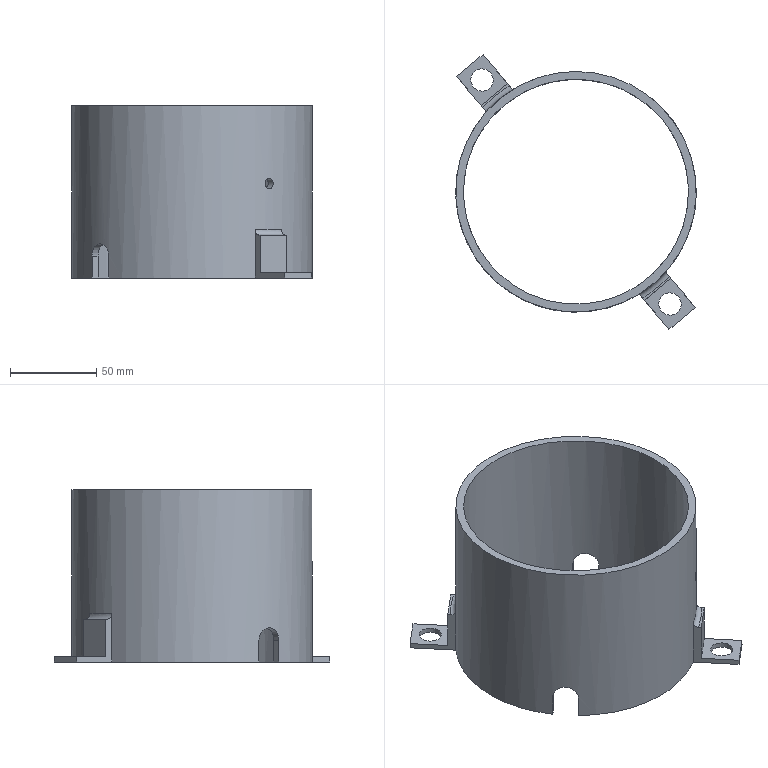Part | NX | features solid 2 | 1 solid | 30 faces | box 139.8 x 159.936 x 100 mm | volume 194922 mm3 | plane 21 | cylinder 7 | torus 2 | commonest cylinder face diameters 13 x2 15 x2 6 x1 130.8 x1 139.8 x1
STEP:
#1=CARTESIAN_POINT('',(1445.459,-595.134,-125.));
#2=VERTEX_POINT('',#1);
#3=CARTESIAN_POINT('',(1449.637,-600.114,-125.));
#4=DIRECTION('',(0.,0.,-1.));
#5=DIRECTION('',(-0.6428,0.766,0.));
#6=AXIS2_PLACEMENT_3D('',#3,#4,#5);
#7=CIRCLE('',#6,6.5);
#8=EDGE_CURVE('',#2,#2,#7,.T.);
#9=ORIENTED_EDGE('',*,*,#8,.F.);
#10=EDGE_LOOP('',(#9));
#11=FACE_BOUND('',#10,.T.);
#12=CARTESIAN_POINT('',(1453.058,-496.074,-125.));
#13=VERTEX_POINT('',#12);
#14=CARTESIAN_POINT('',(1447.129,-581.568,-125.));
#15=VERTEX_POINT('',#14);
#16=CARTESIAN_POINT('',(1395.,-535.,-125.));
#17=DIRECTION('',(0.,0.,-1.));
#18=DIRECTION('',(-0.9659,0.2588,0.));
#19=AXIS2_PLACEMENT_3D('',#16,#17,#18);
#20=CIRCLE('',#19,69.9);
#21=EDGE_CURVE('',#13,#15,#20,.T.);
#22=ORIENTED_EDGE('',*,*,#21,.T.);
#23=CARTESIAN_POINT('',(1464.368,-602.112,-125.));
#24=VERTEX_POINT('',#23);
#25=CARTESIAN_POINT('',(1437.371,-569.939,-125.));
#26=DIRECTION('',(0.6428,-0.766,0.));
#27=VECTOR('',#26,1000.);
#28=LINE('',#25,#27);
#29=EDGE_CURVE('',#15,#24,#28,.T.);
#30=ORIENTED_EDGE('',*,*,#29,.T.);
#31=CARTESIAN_POINT('',(1449.047,-614.968,-125.));
#32=VERTEX_POINT('',#31);
#33=CARTESIAN_POINT('',(1449.047,-614.968,-125.));
#34=DIRECTION('',(0.766,0.6428,0.));
#35=VECTOR('',#34,1000.);
#36=LINE('',#33,#35);
#37=EDGE_CURVE('',#32,#24,#36,.T.);
#38=ORIENTED_EDGE('',*,*,#37,.F.);
#39=CARTESIAN_POINT('',(1431.808,-594.424,-125.));
#40=VERTEX_POINT('',#39);
#41=CARTESIAN_POINT('',(1427.835,-589.689,-125.));
#42=DIRECTION('',(-0.6428,0.766,0.));
#43=VECTOR('',#42,1000.);
#44=LINE('',#41,#43);
#45=EDGE_CURVE('',#32,#40,#44,.T.);
#46=ORIENTED_EDGE('',*,*,#45,.T.);
#47=CARTESIAN_POINT('',(1346.584,-585.417,-125.));
#48=VERTEX_POINT('',#47);
#49=CARTESIAN_POINT('',(1395.,-535.,-125.));
#50=DIRECTION('',(0.,0.,-1.));
#51=DIRECTION('',(-0.9659,0.2588,0.));
#52=AXIS2_PLACEMENT_3D('',#49,#50,#51);
#53=CIRCLE('',#52,69.9);
#54=EDGE_CURVE('',#40,#48,#53,.T.);
#55=ORIENTED_EDGE('',*,*,#54,.T.);
#56=CARTESIAN_POINT('',(1350.052,-582.506,-125.));
#57=VERTEX_POINT('',#56);
#58=CARTESIAN_POINT('',(1399.821,-540.745,-125.));
#59=DIRECTION('',(-0.766,-0.6428,0.));
#60=VECTOR('',#59,1000.);
#61=LINE('',#58,#60);
#62=EDGE_CURVE('',#57,#48,#61,.T.);
#63=ORIENTED_EDGE('',*,*,#62,.F.);
#64=CARTESIAN_POINT('',(1449.59,-498.984,-125.));
#65=VERTEX_POINT('',#64);
#66=CARTESIAN_POINT('',(1395.,-535.,-125.));
#67=DIRECTION('',(0.,0.,-1.));
#68=DIRECTION('',(-0.9659,0.2588,0.));
#69=AXIS2_PLACEMENT_3D('',#66,#67,#68);
#70=CIRCLE('',#69,65.4);
#71=EDGE_CURVE('',#65,#57,#70,.T.);
#72=ORIENTED_EDGE('',*,*,#71,.F.);
#73=CARTESIAN_POINT('',(1399.821,-540.745,-125.));
#74=DIRECTION('',(-0.766,-0.6428,0.));
#75=VECTOR('',#74,1000.);
#76=LINE('',#73,#75);
#77=EDGE_CURVE('',#13,#65,#76,.T.);
#78=ORIENTED_EDGE('',*,*,#77,.F.);
#79=EDGE_LOOP('',(#22,#30,#38,#46,#55,#63,#72,#78));
#80=FACE_BOUND('',#79,.T.);
#81=CARTESIAN_POINT('',(1395.,-535.,-125.));
#82=DIRECTION('',(0.,0.,1.));
#83=DIRECTION('',(-0.6428,0.766,0.));
#84=AXIS2_PLACEMENT_3D('',#81,#82,#83);
#85=PLANE('',#84);
#86=ADVANCED_FACE('',(#11,#80),#85,.F.);
#87=CARTESIAN_POINT('',(1355.094,-471.885,-100.));
#88=VERTEX_POINT('',#87);
#89=CARTESIAN_POINT('',(1356.244,-473.255,-100.));
#90=VERTEX_POINT('',#89);
#91=CARTESIAN_POINT('',(1362.165,-480.311,-100.));
#92=DIRECTION('',(0.6428,-0.766,0.));
#93=VECTOR('',#92,1000.);
#94=LINE('',#91,#93);
#95=EDGE_CURVE('',#88,#90,#94,.T.);
#96=ORIENTED_EDGE('',*,*,#95,.F.);
#97=CARTESIAN_POINT('',(1347.434,-478.313,-100.));
#98=VERTEX_POINT('',#97);
#99=CARTESIAN_POINT('',(1339.773,-484.741,-100.));
#100=DIRECTION('',(0.766,0.6428,0.));
#101=VECTOR('',#100,1000.);
#102=LINE('',#99,#101);
#103=EDGE_CURVE('',#98,#88,#102,.T.);
#104=ORIENTED_EDGE('',*,*,#103,.F.);
#105=CARTESIAN_POINT('',(1348.141,-479.155,-100.));
#106=VERTEX_POINT('',#105);
#107=CARTESIAN_POINT('',(1348.141,-479.155,-100.));
#108=CARTESIAN_POINT('',(1347.905,-478.874,-100.));
#109=CARTESIAN_POINT('',(1347.669,-478.594,-100.));
#110=CARTESIAN_POINT('',(1347.434,-478.313,-100.));
#111=B_SPLINE_CURVE_WITH_KNOTS('',3,(#107,#108,#109,#110),.UNSPECIFIED.,.F.,.F.,(4,4),(0.9,1.),.UNSPECIFIED.);
#112=EDGE_CURVE('',#106,#98,#111,.T.);
#113=ORIENTED_EDGE('',*,*,#112,.F.);
#114=CARTESIAN_POINT('',(1395.,-535.,-100.));
#115=DIRECTION('',(0.,0.,-1.));
#116=DIRECTION('',(-0.9659,0.2588,0.));
#117=AXIS2_PLACEMENT_3D('',#114,#115,#116);
#118=CIRCLE('',#117,72.9);
#119=EDGE_CURVE('',#90,#106,#118,.F.);
#120=ORIENTED_EDGE('',*,*,#119,.F.);
#121=EDGE_LOOP('',(#96,#104,#113,#120));
#122=FACE_BOUND('',#121,.T.);
#123=CARTESIAN_POINT('',(1367.95,-487.206,-100.));
#124=DIRECTION('',(0.,0.,1.));
#125=DIRECTION('',(-0.6428,0.766,0.));
#126=AXIS2_PLACEMENT_3D('',#123,#124,#125);
#127=PLANE('',#126);
#128=ADVANCED_FACE('',(#122),#127,.T.);
#129=CARTESIAN_POINT('',(1434.906,-598.115,-100.));
#130=VERTEX_POINT('',#129);
#131=CARTESIAN_POINT('',(1433.756,-596.745,-100.));
#132=VERTEX_POINT('',#131);
#133=CARTESIAN_POINT('',(1427.835,-589.689,-100.));
#134=DIRECTION('',(-0.6428,0.766,0.));
#135=VECTOR('',#134,1000.);
#136=LINE('',#133,#135);
#137=EDGE_CURVE('',#130,#132,#136,.T.);
#138=ORIENTED_EDGE('',*,*,#137,.F.);
#139=CARTESIAN_POINT('',(1442.566,-591.687,-100.));
#140=VERTEX_POINT('',#139);
#141=CARTESIAN_POINT('',(1450.227,-585.259,-100.));
#142=DIRECTION('',(-0.766,-0.6428,0.));
#143=VECTOR('',#142,1000.);
#144=LINE('',#141,#143);
#145=EDGE_CURVE('',#140,#130,#144,.T.);
#146=ORIENTED_EDGE('',*,*,#145,.F.);
#147=CARTESIAN_POINT('',(1441.859,-590.845,-100.));
#148=VERTEX_POINT('',#147);
#149=CARTESIAN_POINT('',(1441.859,-590.845,-100.));
#150=CARTESIAN_POINT('',(1442.095,-591.126,-100.));
#151=CARTESIAN_POINT('',(1442.331,-591.406,-100.));
#152=CARTESIAN_POINT('',(1442.566,-591.687,-100.));
#153=B_SPLINE_CURVE_WITH_KNOTS('',3,(#149,#150,#151,#152),.UNSPECIFIED.,.F.,.F.,(4,4),(0.9,1.),.UNSPECIFIED.);
#154=EDGE_CURVE('',#148,#140,#153,.T.);
#155=ORIENTED_EDGE('',*,*,#154,.F.);
#156=CARTESIAN_POINT('',(1395.,-535.,-100.));
#157=DIRECTION('',(0.,0.,-1.));
#158=DIRECTION('',(-0.9659,0.2588,0.));
#159=AXIS2_PLACEMENT_3D('',#156,#157,#158);
#160=CIRCLE('',#159,72.9);
#161=EDGE_CURVE('',#132,#148,#160,.F.);
#162=ORIENTED_EDGE('',*,*,#161,.F.);
#163=EDGE_LOOP('',(#138,#146,#155,#162));
#164=FACE_BOUND('',#163,.T.);
#165=CARTESIAN_POINT('',(1427.835,-589.689,-100.));
#166=DIRECTION('',(0.,0.,1.));
#167=DIRECTION('',(-0.6428,0.766,0.));
#168=AXIS2_PLACEMENT_3D('',#165,#166,#167);
#169=PLANE('',#168);
#170=ADVANCED_FACE('',(#164),#169,.T.);
#171=CARTESIAN_POINT('',(1439.646,-588.784,-72.977));
#172=VERTEX_POINT('',#171);
#173=CARTESIAN_POINT('',(1437.891,-590.2,-72.04));
#174=CARTESIAN_POINT('',(1439.626,-588.821,-73.3));
#175=CARTESIAN_POINT('',(1441.483,-587.218,-72.622));
#176=CARTESIAN_POINT('',(1442.407,-586.366,-70.413));
#177=CARTESIAN_POINT('',(1441.913,-586.826,-67.959));
#178=CARTESIAN_POINT('',(1440.255,-588.293,-66.701));
#179=CARTESIAN_POINT('',(1438.356,-589.842,-67.375));
#180=CARTESIAN_POINT('',(1437.353,-590.606,-69.586));
#181=CARTESIAN_POINT('',(1437.891,-590.2,-72.04));
#182=CARTESIAN_POINT('',(1439.626,-588.821,-73.3));
#183=CARTESIAN_POINT('',(1441.483,-587.218,-72.622));
#184=B_SPLINE_CURVE_WITH_KNOTS('',3,(#173,#174,#175,#176,#177,#178,#179,#180,#181,#182,#183),.UNSPECIFIED.,.T.,.F.,(1,1,1,1,1,1,1,1,1,1,1,1,1,1,1),(-0.007035,-0.00469,-0.002345,0.,0.002345,0.00469,0.007035,0.009379,0.01172,0.01407,0.01641,0.01876,0.0211,0.02345,0.02579),.UNSPECIFIED.);
#185=EDGE_CURVE('',#172,#172,#184,.T.);
#186=ORIENTED_EDGE('',*,*,#185,.F.);
#187=EDGE_LOOP('',(#186));
#188=FACE_BOUND('',#187,.T.);
#189=CARTESIAN_POINT('',(1327.482,-516.909,-25.));
#190=VERTEX_POINT('',#189);
#191=CARTESIAN_POINT('',(1395.,-535.,-25.));
#192=DIRECTION('',(0.,0.,-1.));
#193=DIRECTION('',(-0.9659,0.2588,0.));
#194=AXIS2_PLACEMENT_3D('',#191,#192,#193);
#195=CIRCLE('',#194,69.9);
#196=EDGE_CURVE('',#190,#190,#195,.T.);
#197=ORIENTED_EDGE('',*,*,#196,.T.);
#198=EDGE_LOOP('',(#197));
#199=FACE_BOUND('',#198,.T.);
#200=CARTESIAN_POINT('',(1443.416,-484.583,-112.5));
#201=VERTEX_POINT('',#200);
#202=CARTESIAN_POINT('',(1453.058,-496.074,-112.5));
#203=VERTEX_POINT('',#202);
#204=CARTESIAN_POINT('',(1443.416,-484.583,-112.5));
#205=CARTESIAN_POINT('',(1443.416,-484.583,-110.517));
#206=CARTESIAN_POINT('',(1444.616,-485.698,-106.634));
#207=CARTESIAN_POINT('',(1448.619,-489.999,-104.184));
#208=CARTESIAN_POINT('',(1452.168,-494.697,-106.628));
#209=CARTESIAN_POINT('',(1453.058,-496.074,-110.517));
#210=CARTESIAN_POINT('',(1453.058,-496.074,-112.5));
#211=B_SPLINE_CURVE_WITH_KNOTS('',3,(#204,#205,#206,#207,#208,#209,#210),.UNSPECIFIED.,.F.,.F.,(4,1,1,1,4),(0.,0.005865,0.01173,0.0176,0.02346),.UNSPECIFIED.);
#212=EDGE_CURVE('',#201,#203,#211,.T.);
#213=ORIENTED_EDGE('',*,*,#212,.F.);
#214=CARTESIAN_POINT('',(1443.416,-484.583,-125.));
#215=VERTEX_POINT('',#214);
#216=CARTESIAN_POINT('',(1443.416,-484.583,-118.75));
#217=DIRECTION('',(0.,0.,-1.));
#218=VECTOR('',#217,1000.);
#219=LINE('',#216,#218);
#220=EDGE_CURVE('',#215,#201,#219,.F.);
#221=ORIENTED_EDGE('',*,*,#220,.F.);
#222=CARTESIAN_POINT('',(1358.192,-475.576,-125.));
#223=VERTEX_POINT('',#222);
#224=CARTESIAN_POINT('',(1395.,-535.,-125.));
#225=DIRECTION('',(0.,0.,-1.));
#226=DIRECTION('',(-0.9659,0.2588,0.));
#227=AXIS2_PLACEMENT_3D('',#224,#225,#226);
#228=CIRCLE('',#227,69.9);
#229=EDGE_CURVE('',#223,#215,#228,.T.);
#230=ORIENTED_EDGE('',*,*,#229,.F.);
#231=CARTESIAN_POINT('',(1358.192,-475.576,-97.));
#232=VERTEX_POINT('',#231);
#233=CARTESIAN_POINT('',(1358.192,-475.576,-111.));
#234=DIRECTION('',(0.,0.,-1.));
#235=VECTOR('',#234,1000.);
#236=LINE('',#233,#235);
#237=EDGE_CURVE('',#223,#232,#236,.F.);
#238=ORIENTED_EDGE('',*,*,#237,.T.);
#239=CARTESIAN_POINT('',(1342.871,-488.432,-97.));
#240=VERTEX_POINT('',#239);
#241=CARTESIAN_POINT('',(1395.,-535.,-97.));
#242=DIRECTION('',(0.,0.,-1.));
#243=DIRECTION('',(-0.9659,0.2588,0.));
#244=AXIS2_PLACEMENT_3D('',#241,#242,#243);
#245=CIRCLE('',#244,69.9);
#246=EDGE_CURVE('',#240,#232,#245,.T.);
#247=ORIENTED_EDGE('',*,*,#246,.F.);
#248=CARTESIAN_POINT('',(1342.871,-488.432,-125.));
#249=VERTEX_POINT('',#248);
#250=CARTESIAN_POINT('',(1342.871,-488.432,-111.));
#251=DIRECTION('',(0.,0.,-1.));
#252=VECTOR('',#251,1000.);
#253=LINE('',#250,#252);
#254=EDGE_CURVE('',#240,#249,#253,.T.);
#255=ORIENTED_EDGE('',*,*,#254,.T.);
#256=CARTESIAN_POINT('',(1336.942,-573.926,-125.));
#257=VERTEX_POINT('',#256);
#258=CARTESIAN_POINT('',(1395.,-535.,-125.));
#259=DIRECTION('',(0.,0.,-1.));
#260=DIRECTION('',(-0.9659,0.2588,0.));
#261=AXIS2_PLACEMENT_3D('',#258,#259,#260);
#262=CIRCLE('',#261,69.9);
#263=EDGE_CURVE('',#257,#249,#262,.T.);
#264=ORIENTED_EDGE('',*,*,#263,.F.);
#265=CARTESIAN_POINT('',(1336.942,-573.926,-112.5));
#266=VERTEX_POINT('',#265);
#267=CARTESIAN_POINT('',(1336.942,-573.926,-118.75));
#268=DIRECTION('',(0.,0.,-1.));
#269=VECTOR('',#268,1000.);
#270=LINE('',#267,#269);
#271=EDGE_CURVE('',#266,#257,#270,.T.);
#272=ORIENTED_EDGE('',*,*,#271,.F.);
#273=CARTESIAN_POINT('',(1346.584,-585.417,-112.5));
#274=VERTEX_POINT('',#273);
#275=CARTESIAN_POINT('',(1346.584,-585.417,-112.5));
#276=CARTESIAN_POINT('',(1346.584,-585.417,-110.517));
#277=CARTESIAN_POINT('',(1345.384,-584.302,-106.634));
#278=CARTESIAN_POINT('',(1341.381,-580.001,-104.184));
#279=CARTESIAN_POINT('',(1337.832,-575.303,-106.628));
#280=CARTESIAN_POINT('',(1336.942,-573.926,-110.517));
#281=CARTESIAN_POINT('',(1336.942,-573.926,-112.5));
#282=B_SPLINE_CURVE_WITH_KNOTS('',3,(#275,#276,#277,#278,#279,#280,#281),.UNSPECIFIED.,.F.,.F.,(4,1,1,1,4),(0.,0.005865,0.01173,0.0176,0.02346),.UNSPECIFIED.);
#283=EDGE_CURVE('',#274,#266,#282,.T.);
#284=ORIENTED_EDGE('',*,*,#283,.F.);
#285=CARTESIAN_POINT('',(1346.584,-585.417,-118.75));
#286=DIRECTION('',(0.,0.,-1.));
#287=VECTOR('',#286,1000.);
#288=LINE('',#285,#287);
#289=EDGE_CURVE('',#48,#274,#288,.F.);
#290=ORIENTED_EDGE('',*,*,#289,.F.);
#291=ORIENTED_EDGE('',*,*,#54,.F.);
#292=CARTESIAN_POINT('',(1431.808,-594.424,-97.));
#293=VERTEX_POINT('',#292);
#294=CARTESIAN_POINT('',(1431.808,-594.424,-111.));
#295=DIRECTION('',(0.,0.,-1.));
#296=VECTOR('',#295,1000.);
#297=LINE('',#294,#296);
#298=EDGE_CURVE('',#40,#293,#297,.F.);
#299=ORIENTED_EDGE('',*,*,#298,.T.);
#300=CARTESIAN_POINT('',(1447.129,-581.568,-97.));
#301=VERTEX_POINT('',#300);
#302=CARTESIAN_POINT('',(1395.,-535.,-97.));
#303=DIRECTION('',(0.,0.,-1.));
#304=DIRECTION('',(-0.9659,0.2588,0.));
#305=AXIS2_PLACEMENT_3D('',#302,#303,#304);
#306=CIRCLE('',#305,69.9);
#307=EDGE_CURVE('',#301,#293,#306,.T.);
#308=ORIENTED_EDGE('',*,*,#307,.F.);
#309=CARTESIAN_POINT('',(1447.129,-581.568,-111.));
#310=DIRECTION('',(0.,0.,-1.));
#311=VECTOR('',#310,1000.);
#312=LINE('',#309,#311);
#313=EDGE_CURVE('',#301,#15,#312,.T.);
#314=ORIENTED_EDGE('',*,*,#313,.T.);
#315=ORIENTED_EDGE('',*,*,#21,.F.);
#316=CARTESIAN_POINT('',(1453.058,-496.074,-118.75));
#317=DIRECTION('',(0.,0.,-1.));
#318=VECTOR('',#317,1000.);
#319=LINE('',#316,#318);
#320=EDGE_CURVE('',#203,#13,#319,.T.);
#321=ORIENTED_EDGE('',*,*,#320,.F.);
#322=EDGE_LOOP('',(#213,#221,#230,#238,#247,#255,#264,#272,#284,#290,#291,#299,#308,#314,#315,#321));
#323=FACE_BOUND('',#322,.T.);
#324=CARTESIAN_POINT('',(1395.,-535.,-15.));
#325=DIRECTION('',(0.,0.,-1.));
#326=DIRECTION('',(0.6428,-0.766,0.));
#327=AXIS2_PLACEMENT_3D('',#324,#325,#326);
#328=CYLINDRICAL_SURFACE('',#327,69.9);
#329=ADVANCED_FACE('',(#188,#199,#323),#328,.T.);
#330=CARTESIAN_POINT('',(1449.59,-498.984,-112.5));
#331=VERTEX_POINT('',#330);
#332=CARTESIAN_POINT('',(1449.59,-498.984,-118.75));
#333=DIRECTION('',(0.,0.,-1.));
#334=VECTOR('',#333,1000.);
#335=LINE('',#332,#334);
#336=EDGE_CURVE('',#331,#65,#335,.T.);
#337=ORIENTED_EDGE('',*,*,#336,.T.);
#338=ORIENTED_EDGE('',*,*,#71,.T.);
#339=CARTESIAN_POINT('',(1350.052,-582.506,-112.5));
#340=VERTEX_POINT('',#339);
#341=CARTESIAN_POINT('',(1350.052,-582.506,-118.75));
#342=DIRECTION('',(0.,0.,-1.));
#343=VECTOR('',#342,1000.);
#344=LINE('',#341,#343);
#345=EDGE_CURVE('',#57,#340,#344,.F.);
#346=ORIENTED_EDGE('',*,*,#345,.T.);
#347=CARTESIAN_POINT('',(1340.41,-571.016,-112.5));
#348=VERTEX_POINT('',#347);
#349=CARTESIAN_POINT('',(1350.052,-582.506,-112.5));
#350=CARTESIAN_POINT('',(1350.052,-582.506,-110.517));
#351=CARTESIAN_POINT('',(1348.842,-581.4,-106.634));
#352=CARTESIAN_POINT('',(1344.823,-577.113,-104.184));
#353=CARTESIAN_POINT('',(1341.29,-572.401,-106.629));
#354=CARTESIAN_POINT('',(1340.41,-571.016,-110.517));
#355=CARTESIAN_POINT('',(1340.41,-571.016,-112.5));
#356=B_SPLINE_CURVE_WITH_KNOTS('',3,(#349,#350,#351,#352,#353,#354,#355),.UNSPECIFIED.,.F.,.F.,(4,1,1,1,4),(0.,0.005866,0.01173,0.0176,0.02346),.UNSPECIFIED.);
#357=EDGE_CURVE('',#340,#348,#356,.T.);
#358=ORIENTED_EDGE('',*,*,#357,.T.);
#359=CARTESIAN_POINT('',(1340.41,-571.016,-125.));
#360=VERTEX_POINT('',#359);
#361=CARTESIAN_POINT('',(1340.41,-571.016,-118.75));
#362=DIRECTION('',(0.,0.,-1.));
#363=VECTOR('',#362,1000.);
#364=LINE('',#361,#363);
#365=EDGE_CURVE('',#348,#360,#364,.T.);
#366=ORIENTED_EDGE('',*,*,#365,.T.);
#367=CARTESIAN_POINT('',(1439.948,-487.494,-125.));
#368=VERTEX_POINT('',#367);
#369=CARTESIAN_POINT('',(1395.,-535.,-125.));
#370=DIRECTION('',(0.,0.,-1.));
#371=DIRECTION('',(-0.9659,0.2588,0.));
#372=AXIS2_PLACEMENT_3D('',#369,#370,#371);
#373=CIRCLE('',#372,65.4);
#374=EDGE_CURVE('',#360,#368,#373,.T.);
#375=ORIENTED_EDGE('',*,*,#374,.T.);
#376=CARTESIAN_POINT('',(1439.948,-487.494,-112.5));
#377=VERTEX_POINT('',#376);
#378=CARTESIAN_POINT('',(1439.948,-487.494,-118.75));
#379=DIRECTION('',(0.,0.,-1.));
#380=VECTOR('',#379,1000.);
#381=LINE('',#378,#380);
#382=EDGE_CURVE('',#368,#377,#381,.F.);
#383=ORIENTED_EDGE('',*,*,#382,.T.);
#384=CARTESIAN_POINT('',(1439.948,-487.494,-112.5));
#385=CARTESIAN_POINT('',(1439.948,-487.494,-110.517));
#386=CARTESIAN_POINT('',(1441.158,-488.6,-106.634));
#387=CARTESIAN_POINT('',(1445.177,-492.887,-104.184));
#388=CARTESIAN_POINT('',(1448.71,-497.599,-106.629));
#389=CARTESIAN_POINT('',(1449.59,-498.984,-110.517));
#390=CARTESIAN_POINT('',(1449.59,-498.984,-112.5));
#391=B_SPLINE_CURVE_WITH_KNOTS('',3,(#384,#385,#386,#387,#388,#389,#390),.UNSPECIFIED.,.F.,.F.,(4,1,1,1,4),(0.,0.005866,0.01173,0.0176,0.02346),.UNSPECIFIED.);
#392=EDGE_CURVE('',#377,#331,#391,.T.);
#393=ORIENTED_EDGE('',*,*,#392,.T.);
#394=EDGE_LOOP('',(#337,#338,#346,#358,#366,#375,#383,#393));
#395=FACE_BOUND('',#394,.T.);
#396=CARTESIAN_POINT('',(1436.742,-585.347,-72.975));
#397=VERTEX_POINT('',#396);
#398=CARTESIAN_POINT('',(1434.988,-586.757,-72.027));
#399=CARTESIAN_POINT('',(1436.721,-585.386,-73.298));
#400=CARTESIAN_POINT('',(1438.579,-583.779,-72.633));
#401=CARTESIAN_POINT('',(1439.509,-582.916,-70.43));
#402=CARTESIAN_POINT('',(1439.026,-583.369,-67.972));
#403=CARTESIAN_POINT('',(1437.376,-584.836,-66.703));
#404=CARTESIAN_POINT('',(1435.473,-586.385,-67.364));
#405=CARTESIAN_POINT('',(1434.459,-587.154,-69.569));
#406=CARTESIAN_POINT('',(1434.988,-586.757,-72.027));
#407=CARTESIAN_POINT('',(1436.721,-585.386,-73.298));
#408=CARTESIAN_POINT('',(1438.579,-583.779,-72.633));
#409=B_SPLINE_CURVE_WITH_KNOTS('',3,(#398,#399,#400,#401,#402,#403,#404,#405,#406,#407,#408),.UNSPECIFIED.,.T.,.F.,(1,1,1,1,1,1,1,1,1,1,1,1,1,1,1),(-0.007035,-0.00469,-0.002345,0.,0.002345,0.00469,0.007035,0.00938,0.01172,0.01407,0.01641,0.01876,0.0211,0.02345,0.02579),.UNSPECIFIED.);
#410=EDGE_CURVE('',#397,#397,#409,.T.);
#411=ORIENTED_EDGE('',*,*,#410,.T.);
#412=EDGE_LOOP('',(#411));
#413=FACE_BOUND('',#412,.T.);
#414=CARTESIAN_POINT('',(1331.828,-518.073,-25.));
#415=VERTEX_POINT('',#414);
#416=CARTESIAN_POINT('',(1395.,-535.,-25.));
#417=DIRECTION('',(0.,0.,-1.));
#418=DIRECTION('',(-0.9659,0.2588,0.));
#419=AXIS2_PLACEMENT_3D('',#416,#417,#418);
#420=CIRCLE('',#419,65.4);
#421=EDGE_CURVE('',#415,#415,#420,.T.);
#422=ORIENTED_EDGE('',*,*,#421,.F.);
#423=EDGE_LOOP('',(#422));
#424=FACE_BOUND('',#423,.T.);
#425=CARTESIAN_POINT('',(1395.,-535.,-15.));
#426=DIRECTION('',(0.,0.,-1.));
#427=DIRECTION('',(0.6428,-0.766,0.));
#428=AXIS2_PLACEMENT_3D('',#425,#426,#427);
#429=CYLINDRICAL_SURFACE('',#428,65.4);
#430=ADVANCED_FACE('',(#395,#413,#424),#429,.F.);
#431=ORIENTED_EDGE('',*,*,#421,.T.);
#432=EDGE_LOOP('',(#431));
#433=FACE_BOUND('',#432,.T.);
#434=ORIENTED_EDGE('',*,*,#196,.F.);
#435=EDGE_LOOP('',(#434));
#436=FACE_BOUND('',#435,.T.);
#437=CARTESIAN_POINT('',(1395.,-535.,-25.));
#438=DIRECTION('',(0.,0.,1.));
#439=DIRECTION('',(-0.6428,0.766,0.));
#440=AXIS2_PLACEMENT_3D('',#437,#438,#439);
#441=PLANE('',#440);
#442=ADVANCED_FACE('',(#433,#436),#441,.T.);
#443=ORIENTED_EDGE('',*,*,#374,.F.);
#444=CARTESIAN_POINT('',(1390.179,-529.255,-125.));
#445=DIRECTION('',(0.766,0.6428,0.));
#446=VECTOR('',#445,1000.);
#447=LINE('',#444,#446);
#448=EDGE_CURVE('',#257,#360,#447,.T.);
#449=ORIENTED_EDGE('',*,*,#448,.F.);
#450=ORIENTED_EDGE('',*,*,#263,.T.);
#451=CARTESIAN_POINT('',(1325.632,-467.888,-125.));
#452=VERTEX_POINT('',#451);
#453=CARTESIAN_POINT('',(1352.629,-500.061,-125.));
#454=DIRECTION('',(-0.6428,0.766,0.));
#455=VECTOR('',#454,1000.);
#456=LINE('',#453,#455);
#457=EDGE_CURVE('',#249,#452,#456,.T.);
#458=ORIENTED_EDGE('',*,*,#457,.T.);
#459=CARTESIAN_POINT('',(1340.953,-455.032,-125.));
#460=VERTEX_POINT('',#459);
#461=CARTESIAN_POINT('',(1340.953,-455.032,-125.));
#462=DIRECTION('',(-0.766,-0.6428,0.));
#463=VECTOR('',#462,1000.);
#464=LINE('',#461,#463);
#465=EDGE_CURVE('',#460,#452,#464,.T.);
#466=ORIENTED_EDGE('',*,*,#465,.F.);
#467=CARTESIAN_POINT('',(1362.165,-480.311,-125.));
#468=DIRECTION('',(0.6428,-0.766,0.));
#469=VECTOR('',#468,1000.);
#470=LINE('',#467,#469);
#471=EDGE_CURVE('',#460,#223,#470,.T.);
#472=ORIENTED_EDGE('',*,*,#471,.T.);
#473=ORIENTED_EDGE('',*,*,#229,.T.);
#474=CARTESIAN_POINT('',(1390.179,-529.255,-125.));
#475=DIRECTION('',(0.766,0.6428,0.));
#476=VECTOR('',#475,1000.);
#477=LINE('',#474,#476);
#478=EDGE_CURVE('',#368,#215,#477,.T.);
#479=ORIENTED_EDGE('',*,*,#478,.F.);
#480=EDGE_LOOP('',(#443,#449,#450,#458,#466,#472,#473,#479));
#481=FACE_BOUND('',#480,.T.);
#482=CARTESIAN_POINT('',(1336.185,-464.907,-125.));
#483=VERTEX_POINT('',#482);
#484=CARTESIAN_POINT('',(1340.363,-469.886,-125.));
#485=DIRECTION('',(0.,0.,-1.));
#486=DIRECTION('',(-0.6428,0.766,0.));
#487=AXIS2_PLACEMENT_3D('',#484,#485,#486);
#488=CIRCLE('',#487,6.5);
#489=EDGE_CURVE('',#483,#483,#488,.T.);
#490=ORIENTED_EDGE('',*,*,#489,.F.);
#491=EDGE_LOOP('',(#490));
#492=FACE_BOUND('',#491,.T.);
#493=CARTESIAN_POINT('',(1395.,-535.,-125.));
#494=DIRECTION('',(0.,0.,1.));
#495=DIRECTION('',(-0.6428,0.766,0.));
#496=AXIS2_PLACEMENT_3D('',#493,#494,#495);
#497=PLANE('',#496);
#498=ADVANCED_FACE('',(#481,#492),#497,.F.);
#499=CARTESIAN_POINT('',(1450.227,-585.259,-100.));
#500=VERTEX_POINT('',#499);
#501=CARTESIAN_POINT('',(1450.227,-585.259,-100.));
#502=DIRECTION('',(-0.766,-0.6428,0.));
#503=VECTOR('',#502,1000.);
#504=LINE('',#501,#503);
#505=EDGE_CURVE('',#500,#140,#504,.T.);
#506=ORIENTED_EDGE('',*,*,#505,.F.);
#507=CARTESIAN_POINT('',(1449.077,-583.889,-100.));
#508=VERTEX_POINT('',#507);
#509=CARTESIAN_POINT('',(1437.371,-569.939,-100.));
#510=DIRECTION('',(0.6428,-0.766,0.));
#511=VECTOR('',#510,1000.);
#512=LINE('',#509,#511);
#513=EDGE_CURVE('',#508,#500,#512,.T.);
#514=ORIENTED_EDGE('',*,*,#513,.F.);
#515=CARTESIAN_POINT('',(1395.,-535.,-100.));
#516=DIRECTION('',(0.,0.,-1.));
#517=DIRECTION('',(-0.9659,0.2588,0.));
#518=AXIS2_PLACEMENT_3D('',#515,#516,#517);
#519=CIRCLE('',#518,72.9);
#520=EDGE_CURVE('',#148,#508,#519,.F.);
#521=ORIENTED_EDGE('',*,*,#520,.F.);
#522=ORIENTED_EDGE('',*,*,#154,.T.);
#523=EDGE_LOOP('',(#506,#514,#521,#522));
#524=FACE_BOUND('',#523,.T.);
#525=CARTESIAN_POINT('',(1427.835,-589.689,-100.));
#526=DIRECTION('',(0.,0.,1.));
#527=DIRECTION('',(-0.6428,0.766,0.));
#528=AXIS2_PLACEMENT_3D('',#525,#526,#527);
#529=PLANE('',#528);
#530=ADVANCED_FACE('',(#524),#529,.T.);
#531=ORIENTED_EDGE('',*,*,#45,.F.);
#532=CARTESIAN_POINT('',(1449.047,-614.968,-122.));
#533=VERTEX_POINT('',#532);
#534=CARTESIAN_POINT('',(1449.047,-614.968,-122.));
#535=DIRECTION('',(0.,0.,-1.));
#536=VECTOR('',#535,1000.);
#537=LINE('',#534,#536);
#538=EDGE_CURVE('',#533,#32,#537,.T.);
#539=ORIENTED_EDGE('',*,*,#538,.F.);
#540=CARTESIAN_POINT('',(1434.906,-598.115,-122.));
#541=VERTEX_POINT('',#540);
#542=CARTESIAN_POINT('',(1427.835,-589.689,-122.));
#543=DIRECTION('',(0.6428,-0.766,0.));
#544=VECTOR('',#543,1000.);
#545=LINE('',#542,#544);
#546=EDGE_CURVE('',#541,#533,#545,.T.);
#547=ORIENTED_EDGE('',*,*,#546,.F.);
#548=CARTESIAN_POINT('',(1434.906,-598.115,-100.));
#549=DIRECTION('',(0.,0.,-1.));
#550=VECTOR('',#549,1000.);
#551=LINE('',#548,#550);
#552=EDGE_CURVE('',#130,#541,#551,.T.);
#553=ORIENTED_EDGE('',*,*,#552,.F.);
#554=ORIENTED_EDGE('',*,*,#137,.T.);
#555=CARTESIAN_POINT('',(1431.808,-594.424,-97.));
#556=CARTESIAN_POINT('',(1431.808,-594.424,-97.796));
#557=CARTESIAN_POINT('',(1432.237,-594.935,-99.353));
#558=CARTESIAN_POINT('',(1433.244,-596.135,-100.));
#559=CARTESIAN_POINT('',(1433.756,-596.745,-100.));
#560=B_SPLINE_CURVE_WITH_KNOTS('',3,(#555,#556,#557,#558,#559),.UNSPECIFIED.,.F.,.F.,(4,1,4),(0.,0.002355,0.00471),.UNSPECIFIED.);
#561=EDGE_CURVE('',#293,#132,#560,.T.);
#562=ORIENTED_EDGE('',*,*,#561,.F.);
#563=ORIENTED_EDGE('',*,*,#298,.F.);
#564=EDGE_LOOP('',(#531,#539,#547,#553,#554,#562,#563));
#565=FACE_BOUND('',#564,.T.);
#566=CARTESIAN_POINT('',(1427.835,-589.689,-100.));
#567=DIRECTION('',(0.766,0.6428,0.));
#568=DIRECTION('',(0.6428,-0.766,0.));
#569=AXIS2_PLACEMENT_3D('',#566,#567,#568);
#570=PLANE('',#569);
#571=ADVANCED_FACE('',(#565),#570,.F.);
#572=ORIENTED_EDGE('',*,*,#513,.T.);
#573=CARTESIAN_POINT('',(1450.227,-585.259,-122.));
#574=VERTEX_POINT('',#573);
#575=CARTESIAN_POINT('',(1450.227,-585.259,-100.));
#576=DIRECTION('',(0.,0.,-1.));
#577=VECTOR('',#576,1000.);
#578=LINE('',#575,#577);
#579=EDGE_CURVE('',#500,#574,#578,.T.);
#580=ORIENTED_EDGE('',*,*,#579,.T.);
#581=CARTESIAN_POINT('',(1464.368,-602.112,-122.));
#582=VERTEX_POINT('',#581);
#583=CARTESIAN_POINT('',(1457.297,-593.686,-122.));
#584=DIRECTION('',(-0.6428,0.766,0.));
#585=VECTOR('',#584,1000.);
#586=LINE('',#583,#585);
#587=EDGE_CURVE('',#582,#574,#586,.T.);
#588=ORIENTED_EDGE('',*,*,#587,.F.);
#589=CARTESIAN_POINT('',(1464.368,-602.112,-100.));
#590=DIRECTION('',(0.,0.,-1.));
#591=VECTOR('',#590,1000.);
#592=LINE('',#589,#591);
#593=EDGE_CURVE('',#582,#24,#592,.T.);
#594=ORIENTED_EDGE('',*,*,#593,.T.);
#595=ORIENTED_EDGE('',*,*,#29,.F.);
#596=ORIENTED_EDGE('',*,*,#313,.F.);
#597=CARTESIAN_POINT('',(1449.077,-583.889,-100.));
#598=CARTESIAN_POINT('',(1448.565,-583.279,-100.));
#599=CARTESIAN_POINT('',(1447.56,-582.081,-99.356));
#600=CARTESIAN_POINT('',(1447.129,-581.568,-97.796));
#601=CARTESIAN_POINT('',(1447.129,-581.568,-97.));
#602=B_SPLINE_CURVE_WITH_KNOTS('',3,(#597,#598,#599,#600,#601),.UNSPECIFIED.,.F.,.F.,(4,1,4),(0.,0.002355,0.00471),.UNSPECIFIED.);
#603=EDGE_CURVE('',#508,#301,#602,.T.);
#604=ORIENTED_EDGE('',*,*,#603,.F.);
#605=EDGE_LOOP('',(#572,#580,#588,#594,#595,#596,#604));
#606=FACE_BOUND('',#605,.T.);
#607=CARTESIAN_POINT('',(1437.371,-569.939,-100.));
#608=DIRECTION('',(-0.766,-0.6428,0.));
#609=DIRECTION('',(-0.6428,0.766,0.));
#610=AXIS2_PLACEMENT_3D('',#607,#608,#609);
#611=PLANE('',#610);
#612=ADVANCED_FACE('',(#606),#611,.F.);
#613=ORIENTED_EDGE('',*,*,#579,.F.);
#614=ORIENTED_EDGE('',*,*,#505,.T.);
#615=ORIENTED_EDGE('',*,*,#145,.T.);
#616=ORIENTED_EDGE('',*,*,#552,.T.);
#617=CARTESIAN_POINT('',(1450.227,-585.259,-122.));
#618=DIRECTION('',(-0.766,-0.6428,0.));
#619=VECTOR('',#618,1000.);
#620=LINE('',#617,#619);
#621=EDGE_CURVE('',#574,#541,#620,.T.);
#622=ORIENTED_EDGE('',*,*,#621,.F.);
#623=EDGE_LOOP('',(#613,#614,#615,#616,#622));
#624=FACE_BOUND('',#623,.T.);
#625=CARTESIAN_POINT('',(1450.227,-585.259,-100.));
#626=DIRECTION('',(-0.6428,0.766,0.));
#627=DIRECTION('',(0.,0.,-1.));
#628=AXIS2_PLACEMENT_3D('',#625,#626,#627);
#629=PLANE('',#628);
#630=ADVANCED_FACE('',(#624),#629,.F.);
#631=CARTESIAN_POINT('',(1339.773,-484.741,-100.));
#632=VERTEX_POINT('',#631);
#633=CARTESIAN_POINT('',(1339.773,-484.741,-100.));
#634=DIRECTION('',(0.766,0.6428,0.));
#635=VECTOR('',#634,1000.);
#636=LINE('',#633,#635);
#637=EDGE_CURVE('',#632,#98,#636,.T.);
#638=ORIENTED_EDGE('',*,*,#637,.F.);
#639=CARTESIAN_POINT('',(1340.923,-486.111,-100.));
#640=VERTEX_POINT('',#639);
#641=CARTESIAN_POINT('',(1352.629,-500.061,-100.));
#642=DIRECTION('',(-0.6428,0.766,0.));
#643=VECTOR('',#642,1000.);
#644=LINE('',#641,#643);
#645=EDGE_CURVE('',#640,#632,#644,.T.);
#646=ORIENTED_EDGE('',*,*,#645,.F.);
#647=CARTESIAN_POINT('',(1395.,-535.,-100.));
#648=DIRECTION('',(0.,0.,-1.));
#649=DIRECTION('',(-0.9659,0.2588,0.));
#650=AXIS2_PLACEMENT_3D('',#647,#648,#649);
#651=CIRCLE('',#650,72.9);
#652=EDGE_CURVE('',#106,#640,#651,.F.);
#653=ORIENTED_EDGE('',*,*,#652,.F.);
#654=ORIENTED_EDGE('',*,*,#112,.T.);
#655=EDGE_LOOP('',(#638,#646,#653,#654));
#656=FACE_BOUND('',#655,.T.);
#657=CARTESIAN_POINT('',(1367.95,-487.206,-100.));
#658=DIRECTION('',(0.,0.,1.));
#659=DIRECTION('',(-0.6428,0.766,0.));
#660=AXIS2_PLACEMENT_3D('',#657,#658,#659);
#661=PLANE('',#660);
#662=ADVANCED_FACE('',(#656),#661,.T.);
#663=ORIENTED_EDGE('',*,*,#471,.F.);
#664=CARTESIAN_POINT('',(1340.953,-455.032,-122.));
#665=VERTEX_POINT('',#664);
#666=CARTESIAN_POINT('',(1340.953,-455.032,-122.));
#667=DIRECTION('',(0.,0.,-1.));
#668=VECTOR('',#667,1000.);
#669=LINE('',#666,#668);
#670=EDGE_CURVE('',#665,#460,#669,.T.);
#671=ORIENTED_EDGE('',*,*,#670,.F.);
#672=CARTESIAN_POINT('',(1355.094,-471.885,-122.));
#673=VERTEX_POINT('',#672);
#674=CARTESIAN_POINT('',(1362.165,-480.311,-122.));
#675=DIRECTION('',(-0.6428,0.766,0.));
#676=VECTOR('',#675,1000.);
#677=LINE('',#674,#676);
#678=EDGE_CURVE('',#673,#665,#677,.T.);
#679=ORIENTED_EDGE('',*,*,#678,.F.);
#680=CARTESIAN_POINT('',(1355.094,-471.885,-100.));
#681=DIRECTION('',(0.,0.,-1.));
#682=VECTOR('',#681,1000.);
#683=LINE('',#680,#682);
#684=EDGE_CURVE('',#88,#673,#683,.T.);
#685=ORIENTED_EDGE('',*,*,#684,.F.);
#686=ORIENTED_EDGE('',*,*,#95,.T.);
#687=CARTESIAN_POINT('',(1358.192,-475.576,-97.));
#688=CARTESIAN_POINT('',(1358.192,-475.576,-97.796));
#689=CARTESIAN_POINT('',(1357.763,-475.065,-99.353));
#690=CARTESIAN_POINT('',(1356.756,-473.865,-100.));
#691=CARTESIAN_POINT('',(1356.244,-473.255,-100.));
#692=B_SPLINE_CURVE_WITH_KNOTS('',3,(#687,#688,#689,#690,#691),.UNSPECIFIED.,.F.,.F.,(4,1,4),(0.,0.002355,0.00471),.UNSPECIFIED.);
#693=EDGE_CURVE('',#232,#90,#692,.T.);
#694=ORIENTED_EDGE('',*,*,#693,.F.);
#695=ORIENTED_EDGE('',*,*,#237,.F.);
#696=EDGE_LOOP('',(#663,#671,#679,#685,#686,#694,#695));
#697=FACE_BOUND('',#696,.T.);
#698=CARTESIAN_POINT('',(1362.165,-480.311,-100.));
#699=DIRECTION('',(-0.766,-0.6428,0.));
#700=DIRECTION('',(-0.6428,0.766,0.));
#701=AXIS2_PLACEMENT_3D('',#698,#699,#700);
#702=PLANE('',#701);
#703=ADVANCED_FACE('',(#697),#702,.F.);
#704=ORIENTED_EDGE('',*,*,#645,.T.);
#705=CARTESIAN_POINT('',(1339.773,-484.741,-122.));
#706=VERTEX_POINT('',#705);
#707=CARTESIAN_POINT('',(1339.773,-484.741,-100.));
#708=DIRECTION('',(0.,0.,-1.));
#709=VECTOR('',#708,1000.);
#710=LINE('',#707,#709);
#711=EDGE_CURVE('',#632,#706,#710,.T.);
#712=ORIENTED_EDGE('',*,*,#711,.T.);
#713=CARTESIAN_POINT('',(1325.632,-467.888,-122.));
#714=VERTEX_POINT('',#713);
#715=CARTESIAN_POINT('',(1332.703,-476.314,-122.));
#716=DIRECTION('',(0.6428,-0.766,0.));
#717=VECTOR('',#716,1000.);
#718=LINE('',#715,#717);
#719=EDGE_CURVE('',#714,#706,#718,.T.);
#720=ORIENTED_EDGE('',*,*,#719,.F.);
#721=CARTESIAN_POINT('',(1325.632,-467.888,-100.));
#722=DIRECTION('',(0.,0.,-1.));
#723=VECTOR('',#722,1000.);
#724=LINE('',#721,#723);
#725=EDGE_CURVE('',#714,#452,#724,.T.);
#726=ORIENTED_EDGE('',*,*,#725,.T.);
#727=ORIENTED_EDGE('',*,*,#457,.F.);
#728=ORIENTED_EDGE('',*,*,#254,.F.);
#729=CARTESIAN_POINT('',(1340.923,-486.111,-100.));
#730=CARTESIAN_POINT('',(1341.435,-486.721,-100.));
#731=CARTESIAN_POINT('',(1342.44,-487.919,-99.356));
#732=CARTESIAN_POINT('',(1342.871,-488.432,-97.796));
#733=CARTESIAN_POINT('',(1342.871,-488.432,-97.));
#734=B_SPLINE_CURVE_WITH_KNOTS('',3,(#729,#730,#731,#732,#733),.UNSPECIFIED.,.F.,.F.,(4,1,4),(0.,0.002355,0.00471),.UNSPECIFIED.);
#735=EDGE_CURVE('',#640,#240,#734,.T.);
#736=ORIENTED_EDGE('',*,*,#735,.F.);
#737=EDGE_LOOP('',(#704,#712,#720,#726,#727,#728,#736));
#738=FACE_BOUND('',#737,.T.);
#739=CARTESIAN_POINT('',(1352.629,-500.061,-100.));
#740=DIRECTION('',(0.766,0.6428,0.));
#741=DIRECTION('',(0.,0.,1.));
#742=AXIS2_PLACEMENT_3D('',#739,#740,#741);
#743=PLANE('',#742);
#744=ADVANCED_FACE('',(#738),#743,.F.);
#745=ORIENTED_EDGE('',*,*,#711,.F.);
#746=ORIENTED_EDGE('',*,*,#637,.T.);
#747=ORIENTED_EDGE('',*,*,#103,.T.);
#748=ORIENTED_EDGE('',*,*,#684,.T.);
#749=CARTESIAN_POINT('',(1339.773,-484.741,-122.));
#750=DIRECTION('',(0.766,0.6428,0.));
#751=VECTOR('',#750,1000.);
#752=LINE('',#749,#751);
#753=EDGE_CURVE('',#706,#673,#752,.T.);
#754=ORIENTED_EDGE('',*,*,#753,.F.);
#755=EDGE_LOOP('',(#745,#746,#747,#748,#754));
#756=FACE_BOUND('',#755,.T.);
#757=CARTESIAN_POINT('',(1339.773,-484.741,-100.));
#758=DIRECTION('',(0.6428,-0.766,0.));
#759=DIRECTION('',(0.,0.,1.));
#760=AXIS2_PLACEMENT_3D('',#757,#758,#759);
#761=PLANE('',#760);
#762=ADVANCED_FACE('',(#756),#761,.F.);
#763=ORIENTED_EDGE('',*,*,#465,.T.);
#764=ORIENTED_EDGE('',*,*,#725,.F.);
#765=CARTESIAN_POINT('',(1340.953,-455.032,-122.));
#766=DIRECTION('',(-0.766,-0.6428,0.));
#767=VECTOR('',#766,1000.);
#768=LINE('',#765,#767);
#769=EDGE_CURVE('',#665,#714,#768,.T.);
#770=ORIENTED_EDGE('',*,*,#769,.F.);
#771=ORIENTED_EDGE('',*,*,#670,.T.);
#772=EDGE_LOOP('',(#763,#764,#770,#771));
#773=FACE_BOUND('',#772,.T.);
#774=CARTESIAN_POINT('',(1340.953,-455.032,-122.));
#775=DIRECTION('',(-0.6428,0.766,0.));
#776=DIRECTION('',(0.,0.,-1.));
#777=AXIS2_PLACEMENT_3D('',#774,#775,#776);
#778=PLANE('',#777);
#779=ADVANCED_FACE('',(#773),#778,.T.);
#780=CARTESIAN_POINT('',(1336.185,-464.907,-122.));
#781=VERTEX_POINT('',#780);
#782=CARTESIAN_POINT('',(1340.363,-469.886,-122.));
#783=DIRECTION('',(0.,0.,-1.));
#784=DIRECTION('',(-0.6428,0.766,0.));
#785=AXIS2_PLACEMENT_3D('',#782,#783,#784);
#786=CIRCLE('',#785,6.5);
#787=EDGE_CURVE('',#781,#781,#786,.T.);
#788=ORIENTED_EDGE('',*,*,#787,.F.);
#789=EDGE_LOOP('',(#788));
#790=FACE_BOUND('',#789,.T.);
#791=ORIENTED_EDGE('',*,*,#489,.T.);
#792=EDGE_LOOP('',(#791));
#793=FACE_BOUND('',#792,.T.);
#794=CARTESIAN_POINT('',(1340.363,-469.886,-122.));
#795=DIRECTION('',(0.,0.,-1.));
#796=DIRECTION('',(0.6428,-0.766,0.));
#797=AXIS2_PLACEMENT_3D('',#794,#795,#796);
#798=CYLINDRICAL_SURFACE('',#797,6.5);
#799=ADVANCED_FACE('',(#790,#793),#798,.F.);
#800=ORIENTED_EDGE('',*,*,#769,.T.);
#801=ORIENTED_EDGE('',*,*,#719,.T.);
#802=ORIENTED_EDGE('',*,*,#753,.T.);
#803=ORIENTED_EDGE('',*,*,#678,.T.);
#804=EDGE_LOOP('',(#800,#801,#802,#803));
#805=FACE_BOUND('',#804,.T.);
#806=ORIENTED_EDGE('',*,*,#787,.T.);
#807=EDGE_LOOP('',(#806));
#808=FACE_BOUND('',#807,.T.);
#809=CARTESIAN_POINT('',(1348.023,-463.458,-122.));
#810=DIRECTION('',(0.,0.,1.));
#811=DIRECTION('',(-0.6428,0.766,0.));
#812=AXIS2_PLACEMENT_3D('',#809,#810,#811);
#813=PLANE('',#812);
#814=ADVANCED_FACE('',(#805,#808),#813,.T.);
#815=ORIENTED_EDGE('',*,*,#37,.T.);
#816=ORIENTED_EDGE('',*,*,#593,.F.);
#817=CARTESIAN_POINT('',(1464.368,-602.112,-122.));
#818=DIRECTION('',(0.766,0.6428,0.));
#819=VECTOR('',#818,1000.);
#820=LINE('',#817,#819);
#821=EDGE_CURVE('',#533,#582,#820,.T.);
#822=ORIENTED_EDGE('',*,*,#821,.F.);
#823=ORIENTED_EDGE('',*,*,#538,.T.);
#824=EDGE_LOOP('',(#815,#816,#822,#823));
#825=FACE_BOUND('',#824,.T.);
#826=CARTESIAN_POINT('',(1449.047,-614.968,-122.));
#827=DIRECTION('',(0.6428,-0.766,0.));
#828=DIRECTION('',(0.,0.,1.));
#829=AXIS2_PLACEMENT_3D('',#826,#827,#828);
#830=PLANE('',#829);
#831=ADVANCED_FACE('',(#825),#830,.T.);
#832=CARTESIAN_POINT('',(1445.459,-595.134,-122.));
#833=VERTEX_POINT('',#832);
#834=CARTESIAN_POINT('',(1449.637,-600.114,-122.));
#835=DIRECTION('',(0.,0.,-1.));
#836=DIRECTION('',(-0.6428,0.766,0.));
#837=AXIS2_PLACEMENT_3D('',#834,#835,#836);
#838=CIRCLE('',#837,6.5);
#839=EDGE_CURVE('',#833,#833,#838,.T.);
#840=ORIENTED_EDGE('',*,*,#839,.F.);
#841=EDGE_LOOP('',(#840));
#842=FACE_BOUND('',#841,.T.);
#843=ORIENTED_EDGE('',*,*,#8,.T.);
#844=EDGE_LOOP('',(#843));
#845=FACE_BOUND('',#844,.T.);
#846=CARTESIAN_POINT('',(1449.637,-600.114,-122.));
#847=DIRECTION('',(0.,0.,-1.));
#848=DIRECTION('',(0.6428,-0.766,0.));
#849=AXIS2_PLACEMENT_3D('',#846,#847,#848);
#850=CYLINDRICAL_SURFACE('',#849,6.5);
#851=ADVANCED_FACE('',(#842,#845),#850,.F.);
#852=ORIENTED_EDGE('',*,*,#821,.T.);
#853=ORIENTED_EDGE('',*,*,#587,.T.);
#854=ORIENTED_EDGE('',*,*,#621,.T.);
#855=ORIENTED_EDGE('',*,*,#546,.T.);
#856=EDGE_LOOP('',(#852,#853,#854,#855));
#857=FACE_BOUND('',#856,.T.);
#858=ORIENTED_EDGE('',*,*,#839,.T.);
#859=EDGE_LOOP('',(#858));
#860=FACE_BOUND('',#859,.T.);
#861=CARTESIAN_POINT('',(1457.297,-593.686,-122.));
#862=DIRECTION('',(0.,0.,-1.));
#863=DIRECTION('',(0.6428,-0.766,0.));
#864=AXIS2_PLACEMENT_3D('',#861,#862,#863);
#865=PLANE('',#864);
#866=ADVANCED_FACE('',(#857,#860),#865,.F.);
#867=ORIENTED_EDGE('',*,*,#520,.T.);
#868=ORIENTED_EDGE('',*,*,#603,.T.);
#869=ORIENTED_EDGE('',*,*,#307,.T.);
#870=ORIENTED_EDGE('',*,*,#561,.T.);
#871=ORIENTED_EDGE('',*,*,#161,.T.);
#872=EDGE_LOOP('',(#867,#868,#869,#870,#871));
#873=FACE_BOUND('',#872,.T.);
#874=CARTESIAN_POINT('',(1395.,-535.,-97.));
#875=DIRECTION('',(0.,0.,1.));
#876=DIRECTION('',(-0.9659,0.2588,0.));
#877=AXIS2_PLACEMENT_3D('',#874,#875,#876);
#878=TOROIDAL_SURFACE('',#877,72.9,3.);
#879=ADVANCED_FACE('',(#873),#878,.F.);
#880=ORIENTED_EDGE('',*,*,#652,.T.);
#881=ORIENTED_EDGE('',*,*,#735,.T.);
#882=ORIENTED_EDGE('',*,*,#246,.T.);
#883=ORIENTED_EDGE('',*,*,#693,.T.);
#884=ORIENTED_EDGE('',*,*,#119,.T.);
#885=EDGE_LOOP('',(#880,#881,#882,#883,#884));
#886=FACE_BOUND('',#885,.T.);
#887=CARTESIAN_POINT('',(1395.,-535.,-97.));
#888=DIRECTION('',(0.,0.,1.));
#889=DIRECTION('',(-0.9659,0.2588,0.));
#890=AXIS2_PLACEMENT_3D('',#887,#888,#889);
#891=TOROIDAL_SURFACE('',#890,72.9,3.);
#892=ADVANCED_FACE('',(#886),#891,.F.);
#893=ORIENTED_EDGE('',*,*,#410,.F.);
#894=EDGE_LOOP('',(#893));
#895=FACE_BOUND('',#894,.T.);
#896=ORIENTED_EDGE('',*,*,#185,.T.);
#897=EDGE_LOOP('',(#896));
#898=FACE_BOUND('',#897,.T.);
#899=CARTESIAN_POINT('',(1395.,-535.,-70.));
#900=DIRECTION('',(0.6428,-0.766,0.));
#901=DIRECTION('',(0.,0.,1.));
#902=AXIS2_PLACEMENT_3D('',#899,#900,#901);
#903=CYLINDRICAL_SURFACE('',#902,3.);
#904=ADVANCED_FACE('',(#895,#898),#903,.F.);
#905=CARTESIAN_POINT('',(1399.821,-540.745,-112.5));
#906=DIRECTION('',(0.766,0.6428,0.));
#907=VECTOR('',#906,1000.);
#908=LINE('',#905,#907);
#909=EDGE_CURVE('',#274,#340,#908,.T.);
#910=ORIENTED_EDGE('',*,*,#909,.F.);
#911=ORIENTED_EDGE('',*,*,#283,.T.);
#912=CARTESIAN_POINT('',(1390.179,-529.255,-112.5));
#913=DIRECTION('',(0.766,0.6428,0.));
#914=VECTOR('',#913,1000.);
#915=LINE('',#912,#914);
#916=EDGE_CURVE('',#266,#348,#915,.T.);
#917=ORIENTED_EDGE('',*,*,#916,.T.);
#918=ORIENTED_EDGE('',*,*,#357,.F.);
#919=EDGE_LOOP('',(#910,#911,#917,#918));
#920=FACE_BOUND('',#919,.T.);
#921=CARTESIAN_POINT('',(1395.,-535.,-112.5));
#922=DIRECTION('',(0.766,0.6428,0.));
#923=DIRECTION('',(0.,0.,1.));
#924=AXIS2_PLACEMENT_3D('',#921,#922,#923);
#925=CYLINDRICAL_SURFACE('',#924,7.5);
#926=ADVANCED_FACE('',(#920),#925,.F.);
#927=ORIENTED_EDGE('',*,*,#916,.F.);
#928=ORIENTED_EDGE('',*,*,#271,.T.);
#929=ORIENTED_EDGE('',*,*,#448,.T.);
#930=ORIENTED_EDGE('',*,*,#365,.F.);
#931=EDGE_LOOP('',(#927,#928,#929,#930));
#932=FACE_BOUND('',#931,.T.);
#933=CARTESIAN_POINT('',(1390.179,-529.255,-125.));
#934=DIRECTION('',(-0.6428,0.766,0.));
#935=DIRECTION('',(0.,0.,-1.));
#936=AXIS2_PLACEMENT_3D('',#933,#934,#935);
#937=PLANE('',#936);
#938=ADVANCED_FACE('',(#932),#937,.F.);
#939=ORIENTED_EDGE('',*,*,#62,.T.);
#940=ORIENTED_EDGE('',*,*,#289,.T.);
#941=ORIENTED_EDGE('',*,*,#909,.T.);
#942=ORIENTED_EDGE('',*,*,#345,.F.);
#943=EDGE_LOOP('',(#939,#940,#941,#942));
#944=FACE_BOUND('',#943,.T.);
#945=CARTESIAN_POINT('',(1399.821,-540.745,-125.));
#946=DIRECTION('',(0.6428,-0.766,0.));
#947=DIRECTION('',(0.,0.,1.));
#948=AXIS2_PLACEMENT_3D('',#945,#946,#947);
#949=PLANE('',#948);
#950=ADVANCED_FACE('',(#944),#949,.F.);
#951=CARTESIAN_POINT('',(1390.179,-529.255,-112.5));
#952=DIRECTION('',(-0.766,-0.6428,0.));
#953=VECTOR('',#952,1000.);
#954=LINE('',#951,#953);
#955=EDGE_CURVE('',#201,#377,#954,.T.);
#956=ORIENTED_EDGE('',*,*,#955,.F.);
#957=ORIENTED_EDGE('',*,*,#212,.T.);
#958=CARTESIAN_POINT('',(1399.821,-540.745,-112.5));
#959=DIRECTION('',(-0.766,-0.6428,0.));
#960=VECTOR('',#959,1000.);
#961=LINE('',#958,#960);
#962=EDGE_CURVE('',#203,#331,#961,.T.);
#963=ORIENTED_EDGE('',*,*,#962,.T.);
#964=ORIENTED_EDGE('',*,*,#392,.F.);
#965=EDGE_LOOP('',(#956,#957,#963,#964));
#966=FACE_BOUND('',#965,.T.);
#967=CARTESIAN_POINT('',(1395.,-535.,-112.5));
#968=DIRECTION('',(-0.766,-0.6428,0.));
#969=DIRECTION('',(0.,0.,-1.));
#970=AXIS2_PLACEMENT_3D('',#967,#968,#969);
#971=CYLINDRICAL_SURFACE('',#970,7.5);
#972=ADVANCED_FACE('',(#966),#971,.F.);
#973=ORIENTED_EDGE('',*,*,#962,.F.);
#974=ORIENTED_EDGE('',*,*,#320,.T.);
#975=ORIENTED_EDGE('',*,*,#77,.T.);
#976=ORIENTED_EDGE('',*,*,#336,.F.);
#977=EDGE_LOOP('',(#973,#974,#975,#976));
#978=FACE_BOUND('',#977,.T.);
#979=CARTESIAN_POINT('',(1399.821,-540.745,-125.));
#980=DIRECTION('',(0.6428,-0.766,0.));
#981=DIRECTION('',(0.,0.,1.));
#982=AXIS2_PLACEMENT_3D('',#979,#980,#981);
#983=PLANE('',#982);
#984=ADVANCED_FACE('',(#978),#983,.F.);
#985=ORIENTED_EDGE('',*,*,#478,.T.);
#986=ORIENTED_EDGE('',*,*,#220,.T.);
#987=ORIENTED_EDGE('',*,*,#955,.T.);
#988=ORIENTED_EDGE('',*,*,#382,.F.);
#989=EDGE_LOOP('',(#985,#986,#987,#988));
#990=FACE_BOUND('',#989,.T.);
#991=CARTESIAN_POINT('',(1390.179,-529.255,-125.));
#992=DIRECTION('',(-0.6428,0.766,0.));
#993=DIRECTION('',(0.,0.,-1.));
#994=AXIS2_PLACEMENT_3D('',#991,#992,#993);
#995=PLANE('',#994);
#996=ADVANCED_FACE('',(#990),#995,.F.);
#997=CLOSED_SHELL('',(#86,#128,#170,#329,#430,#442,#498,#530,#571,#612,#630,#662,#703,#744,#762,#779,#799,#814,#831,#851,#866,#879,#892,#904,#926,#938,#950,#972,#984,#996));
#998=MANIFOLD_SOLID_BREP('',#997);
#999=(LENGTH_UNIT()NAMED_UNIT(*)SI_UNIT(.MILLI.,.METRE.));
#1000=UNCERTAINTY_MEASURE_WITH_UNIT(LENGTH_MEASURE(0.0508),#999,'','');
#1001=(NAMED_UNIT(*)PLANE_ANGLE_UNIT()SI_UNIT($,.RADIAN.));
#1002=(NAMED_UNIT(*)SI_UNIT($,.STERADIAN.)SOLID_ANGLE_UNIT());
#1003=(GEOMETRIC_REPRESENTATION_CONTEXT(3)GLOBAL_UNCERTAINTY_ASSIGNED_CONTEXT((#1000))GLOBAL_UNIT_ASSIGNED_CONTEXT((#999,#1001,#1002))REPRESENTATION_CONTEXT('',''));
#1004=ADVANCED_BREP_SHAPE_REPRESENTATION('',(#998),#1003);